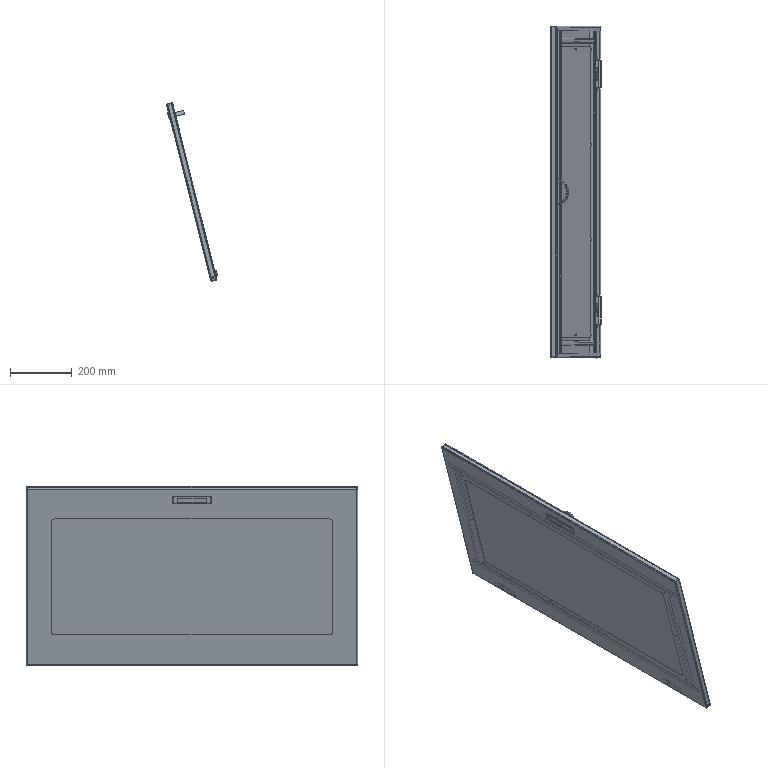Part | NX | features BREP 10 | 12 solids | 594 faces | box 164.614 x 1078 x 580.226 mm | volume 2987115 mm3 | plane 296 | cylinder 216 | cone 48 | torus 18 | spline 16 | commonest cylinder face diameters 7 x38 5 x24 4 x20 5.8 x20 12 x18 8 x16